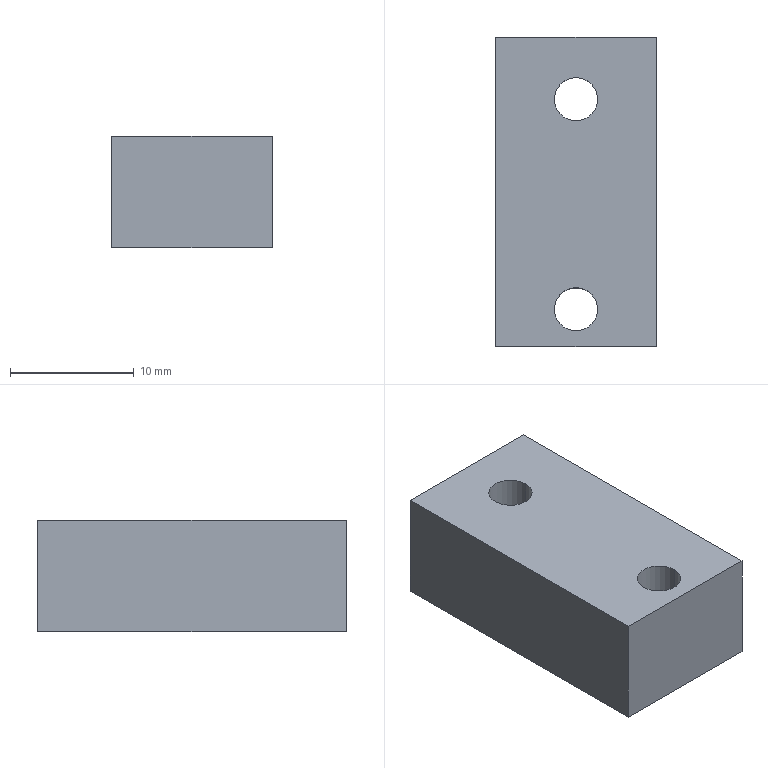Part | SolidWorks | features BaseBody 1 | 1 solid | 10 faces | box 13 x 25 x 9 mm | volume 2752 mm3 | plane 6 | cylinder 4 | commonest cylinder face diameters 3.5 x4
STEP:
#1=CARTESIAN_POINT('',(-21.75,14.,0.));
#2=VERTEX_POINT('',#1);
#3=CARTESIAN_POINT('',(-18.25,14.,0.));
#4=VERTEX_POINT('',#3);
#5=CARTESIAN_POINT('',(-20.,14.,0.));
#6=DIRECTION('',(0.,0.,1.));
#7=DIRECTION('',(1.,0.,0.));
#8=AXIS2_PLACEMENT_3D('',#5,#6,#7);
#9=CIRCLE('',#8,1.75);
#10=EDGE_CURVE('',#2,#4,#9,.T.);
#11=ORIENTED_EDGE('',*,*,#10,.F.);
#12=CARTESIAN_POINT('',(-21.75,14.,9.));
#13=VERTEX_POINT('',#12);
#14=CARTESIAN_POINT('',(-21.75,14.,-20.58));
#15=DIRECTION('',(0.,0.,1.));
#16=VECTOR('',#15,1000.);
#17=LINE('',#14,#16);
#18=EDGE_CURVE('',#2,#13,#17,.T.);
#19=ORIENTED_EDGE('',*,*,#18,.T.);
#20=CARTESIAN_POINT('',(-18.25,14.,9.));
#21=VERTEX_POINT('',#20);
#22=CARTESIAN_POINT('',(-20.,14.,9.));
#23=DIRECTION('',(0.,0.,-1.));
#24=DIRECTION('',(1.,0.,0.));
#25=AXIS2_PLACEMENT_3D('',#22,#23,#24);
#26=CIRCLE('',#25,1.75);
#27=EDGE_CURVE('',#21,#13,#26,.T.);
#28=ORIENTED_EDGE('',*,*,#27,.F.);
#29=CARTESIAN_POINT('',(-18.25,14.,-20.58));
#30=DIRECTION('',(0.,0.,1.));
#31=VECTOR('',#30,1000.);
#32=LINE('',#29,#31);
#33=EDGE_CURVE('',#4,#21,#32,.T.);
#34=ORIENTED_EDGE('',*,*,#33,.F.);
#35=EDGE_LOOP('',(#11,#19,#28,#34));
#36=FACE_OUTER_BOUND('',#35,.T.);
#37=CARTESIAN_POINT('',(-20.,14.,-20.58));
#38=DIRECTION('',(0.,0.,1.));
#39=DIRECTION('',(1.,0.,0.));
#40=AXIS2_PLACEMENT_3D('',#37,#38,#39);
#41=CYLINDRICAL_SURFACE('',#40,1.75);
#42=ADVANCED_FACE('',(#36),#41,.F.);
#43=CARTESIAN_POINT('',(-21.75,-3.,0.));
#44=VERTEX_POINT('',#43);
#45=CARTESIAN_POINT('',(-18.25,-3.,0.));
#46=VERTEX_POINT('',#45);
#47=CARTESIAN_POINT('',(-20.,-3.,0.));
#48=DIRECTION('',(0.,0.,1.));
#49=DIRECTION('',(1.,0.,0.));
#50=AXIS2_PLACEMENT_3D('',#47,#48,#49);
#51=CIRCLE('',#50,1.75);
#52=EDGE_CURVE('',#44,#46,#51,.T.);
#53=ORIENTED_EDGE('',*,*,#52,.F.);
#54=CARTESIAN_POINT('',(-21.75,-3.,9.));
#55=VERTEX_POINT('',#54);
#56=CARTESIAN_POINT('',(-21.75,-3.,-20.58));
#57=DIRECTION('',(0.,0.,1.));
#58=VECTOR('',#57,1000.);
#59=LINE('',#56,#58);
#60=EDGE_CURVE('',#44,#55,#59,.T.);
#61=ORIENTED_EDGE('',*,*,#60,.T.);
#62=CARTESIAN_POINT('',(-18.25,-3.,9.));
#63=VERTEX_POINT('',#62);
#64=CARTESIAN_POINT('',(-20.,-3.,9.));
#65=DIRECTION('',(0.,0.,-1.));
#66=DIRECTION('',(1.,0.,0.));
#67=AXIS2_PLACEMENT_3D('',#64,#65,#66);
#68=CIRCLE('',#67,1.75);
#69=EDGE_CURVE('',#63,#55,#68,.T.);
#70=ORIENTED_EDGE('',*,*,#69,.F.);
#71=CARTESIAN_POINT('',(-18.25,-3.,-20.58));
#72=DIRECTION('',(0.,0.,1.));
#73=VECTOR('',#72,1000.);
#74=LINE('',#71,#73);
#75=EDGE_CURVE('',#46,#63,#74,.T.);
#76=ORIENTED_EDGE('',*,*,#75,.F.);
#77=EDGE_LOOP('',(#53,#61,#70,#76));
#78=FACE_OUTER_BOUND('',#77,.T.);
#79=CARTESIAN_POINT('',(-20.,-3.,-20.58));
#80=DIRECTION('',(0.,0.,1.));
#81=DIRECTION('',(1.,0.,0.));
#82=AXIS2_PLACEMENT_3D('',#79,#80,#81);
#83=CYLINDRICAL_SURFACE('',#82,1.75);
#84=ADVANCED_FACE('',(#78),#83,.F.);
#85=ORIENTED_EDGE('',*,*,#27,.T.);
#86=CARTESIAN_POINT('',(-20.,14.,9.));
#87=DIRECTION('',(0.,0.,-1.));
#88=DIRECTION('',(1.,0.,0.));
#89=AXIS2_PLACEMENT_3D('',#86,#87,#88);
#90=CIRCLE('',#89,1.75);
#91=EDGE_CURVE('',#13,#21,#90,.T.);
#92=ORIENTED_EDGE('',*,*,#91,.T.);
#93=EDGE_LOOP('',(#85,#92));
#94=FACE_BOUND('',#93,.T.);
#95=ORIENTED_EDGE('',*,*,#69,.T.);
#96=CARTESIAN_POINT('',(-20.,-3.,9.));
#97=DIRECTION('',(0.,0.,-1.));
#98=DIRECTION('',(1.,0.,0.));
#99=AXIS2_PLACEMENT_3D('',#96,#97,#98);
#100=CIRCLE('',#99,1.75);
#101=EDGE_CURVE('',#55,#63,#100,.T.);
#102=ORIENTED_EDGE('',*,*,#101,.T.);
#103=EDGE_LOOP('',(#95,#102));
#104=FACE_BOUND('',#103,.T.);
#105=CARTESIAN_POINT('',(-13.5,-6.,9.));
#106=VERTEX_POINT('',#105);
#107=CARTESIAN_POINT('',(-13.5,19.,9.));
#108=VERTEX_POINT('',#107);
#109=CARTESIAN_POINT('',(-13.5,6.5,9.));
#110=DIRECTION('',(0.,1.,0.));
#111=VECTOR('',#110,1000.);
#112=LINE('',#109,#111);
#113=EDGE_CURVE('',#106,#108,#112,.T.);
#114=ORIENTED_EDGE('',*,*,#113,.T.);
#115=CARTESIAN_POINT('',(-26.5,19.,9.));
#116=VERTEX_POINT('',#115);
#117=CARTESIAN_POINT('',(-20.,19.,9.));
#118=DIRECTION('',(-1.,0.,0.));
#119=VECTOR('',#118,1000.);
#120=LINE('',#117,#119);
#121=EDGE_CURVE('',#108,#116,#120,.T.);
#122=ORIENTED_EDGE('',*,*,#121,.T.);
#123=CARTESIAN_POINT('',(-26.5,-6.,9.));
#124=VERTEX_POINT('',#123);
#125=CARTESIAN_POINT('',(-26.5,6.5,9.));
#126=DIRECTION('',(0.,-1.,0.));
#127=VECTOR('',#126,1000.);
#128=LINE('',#125,#127);
#129=EDGE_CURVE('',#116,#124,#128,.T.);
#130=ORIENTED_EDGE('',*,*,#129,.T.);
#131=CARTESIAN_POINT('',(-20.,-6.,9.));
#132=DIRECTION('',(1.,0.,0.));
#133=VECTOR('',#132,1000.);
#134=LINE('',#131,#133);
#135=EDGE_CURVE('',#124,#106,#134,.T.);
#136=ORIENTED_EDGE('',*,*,#135,.T.);
#137=EDGE_LOOP('',(#114,#122,#130,#136));
#138=FACE_OUTER_BOUND('',#137,.T.);
#139=CARTESIAN_POINT('',(-20.,6.5,9.));
#140=DIRECTION('',(0.,0.,1.));
#141=DIRECTION('',(1.,0.,0.));
#142=AXIS2_PLACEMENT_3D('',#139,#140,#141);
#143=PLANE('',#142);
#144=ADVANCED_FACE('',(#94,#104,#138),#143,.T.);
#145=ORIENTED_EDGE('',*,*,#18,.F.);
#146=CARTESIAN_POINT('',(-20.,14.,0.));
#147=DIRECTION('',(0.,0.,1.));
#148=DIRECTION('',(1.,0.,0.));
#149=AXIS2_PLACEMENT_3D('',#146,#147,#148);
#150=CIRCLE('',#149,1.75);
#151=EDGE_CURVE('',#4,#2,#150,.T.);
#152=ORIENTED_EDGE('',*,*,#151,.F.);
#153=ORIENTED_EDGE('',*,*,#33,.T.);
#154=ORIENTED_EDGE('',*,*,#91,.F.);
#155=EDGE_LOOP('',(#145,#152,#153,#154));
#156=FACE_OUTER_BOUND('',#155,.T.);
#157=CARTESIAN_POINT('',(-20.,14.,-20.58));
#158=DIRECTION('',(0.,0.,1.));
#159=DIRECTION('',(1.,0.,0.));
#160=AXIS2_PLACEMENT_3D('',#157,#158,#159);
#161=CYLINDRICAL_SURFACE('',#160,1.75);
#162=ADVANCED_FACE('',(#156),#161,.F.);
#163=ORIENTED_EDGE('',*,*,#60,.F.);
#164=CARTESIAN_POINT('',(-20.,-3.,0.));
#165=DIRECTION('',(0.,0.,1.));
#166=DIRECTION('',(1.,0.,0.));
#167=AXIS2_PLACEMENT_3D('',#164,#165,#166);
#168=CIRCLE('',#167,1.75);
#169=EDGE_CURVE('',#46,#44,#168,.T.);
#170=ORIENTED_EDGE('',*,*,#169,.F.);
#171=ORIENTED_EDGE('',*,*,#75,.T.);
#172=ORIENTED_EDGE('',*,*,#101,.F.);
#173=EDGE_LOOP('',(#163,#170,#171,#172));
#174=FACE_OUTER_BOUND('',#173,.T.);
#175=CARTESIAN_POINT('',(-20.,-3.,-20.58));
#176=DIRECTION('',(0.,0.,1.));
#177=DIRECTION('',(1.,0.,0.));
#178=AXIS2_PLACEMENT_3D('',#175,#176,#177);
#179=CYLINDRICAL_SURFACE('',#178,1.75);
#180=ADVANCED_FACE('',(#174),#179,.F.);
#181=CARTESIAN_POINT('',(-13.5,19.,0.));
#182=VERTEX_POINT('',#181);
#183=CARTESIAN_POINT('',(-26.5,19.,0.));
#184=VERTEX_POINT('',#183);
#185=CARTESIAN_POINT('',(-26.5,19.,0.));
#186=DIRECTION('',(-1.,0.,0.));
#187=VECTOR('',#186,1000.);
#188=LINE('',#185,#187);
#189=EDGE_CURVE('',#182,#184,#188,.T.);
#190=ORIENTED_EDGE('',*,*,#189,.T.);
#191=CARTESIAN_POINT('',(-26.5,19.,0.));
#192=DIRECTION('',(0.,0.,1.));
#193=VECTOR('',#192,1000.);
#194=LINE('',#191,#193);
#195=EDGE_CURVE('',#184,#116,#194,.T.);
#196=ORIENTED_EDGE('',*,*,#195,.T.);
#197=ORIENTED_EDGE('',*,*,#121,.F.);
#198=CARTESIAN_POINT('',(-13.5,19.,0.));
#199=DIRECTION('',(0.,0.,-1.));
#200=VECTOR('',#199,1000.);
#201=LINE('',#198,#200);
#202=EDGE_CURVE('',#108,#182,#201,.T.);
#203=ORIENTED_EDGE('',*,*,#202,.T.);
#204=EDGE_LOOP('',(#190,#196,#197,#203));
#205=FACE_OUTER_BOUND('',#204,.T.);
#206=CARTESIAN_POINT('',(-26.5,19.,0.));
#207=DIRECTION('',(0.,1.,0.));
#208=DIRECTION('',(0.,0.,1.));
#209=AXIS2_PLACEMENT_3D('',#206,#207,#208);
#210=PLANE('',#209);
#211=ADVANCED_FACE('',(#205),#210,.T.);
#212=CARTESIAN_POINT('',(-13.5,-6.,0.));
#213=VERTEX_POINT('',#212);
#214=CARTESIAN_POINT('',(-13.5,19.,0.));
#215=DIRECTION('',(0.,1.,0.));
#216=VECTOR('',#215,1000.);
#217=LINE('',#214,#216);
#218=EDGE_CURVE('',#213,#182,#217,.T.);
#219=ORIENTED_EDGE('',*,*,#218,.T.);
#220=ORIENTED_EDGE('',*,*,#202,.F.);
#221=ORIENTED_EDGE('',*,*,#113,.F.);
#222=CARTESIAN_POINT('',(-13.5,-6.,0.));
#223=DIRECTION('',(0.,0.,-1.));
#224=VECTOR('',#223,1000.);
#225=LINE('',#222,#224);
#226=EDGE_CURVE('',#106,#213,#225,.T.);
#227=ORIENTED_EDGE('',*,*,#226,.T.);
#228=EDGE_LOOP('',(#219,#220,#221,#227));
#229=FACE_OUTER_BOUND('',#228,.T.);
#230=CARTESIAN_POINT('',(-13.5,19.,0.));
#231=DIRECTION('',(1.,0.,0.));
#232=DIRECTION('',(0.,0.,-1.));
#233=AXIS2_PLACEMENT_3D('',#230,#231,#232);
#234=PLANE('',#233);
#235=ADVANCED_FACE('',(#229),#234,.T.);
#236=CARTESIAN_POINT('',(-26.5,-6.,0.));
#237=VERTEX_POINT('',#236);
#238=CARTESIAN_POINT('',(-13.5,-6.,0.));
#239=DIRECTION('',(1.,0.,0.));
#240=VECTOR('',#239,1000.);
#241=LINE('',#238,#240);
#242=EDGE_CURVE('',#237,#213,#241,.T.);
#243=ORIENTED_EDGE('',*,*,#242,.T.);
#244=ORIENTED_EDGE('',*,*,#226,.F.);
#245=ORIENTED_EDGE('',*,*,#135,.F.);
#246=CARTESIAN_POINT('',(-26.5,-6.,0.));
#247=DIRECTION('',(0.,0.,-1.));
#248=VECTOR('',#247,1000.);
#249=LINE('',#246,#248);
#250=EDGE_CURVE('',#124,#237,#249,.T.);
#251=ORIENTED_EDGE('',*,*,#250,.T.);
#252=EDGE_LOOP('',(#243,#244,#245,#251));
#253=FACE_OUTER_BOUND('',#252,.T.);
#254=CARTESIAN_POINT('',(-13.5,-6.,0.));
#255=DIRECTION('',(0.,-1.,0.));
#256=DIRECTION('',(0.,0.,-1.));
#257=AXIS2_PLACEMENT_3D('',#254,#255,#256);
#258=PLANE('',#257);
#259=ADVANCED_FACE('',(#253),#258,.T.);
#260=CARTESIAN_POINT('',(-26.5,-6.,0.));
#261=DIRECTION('',(0.,-1.,0.));
#262=VECTOR('',#261,1000.);
#263=LINE('',#260,#262);
#264=EDGE_CURVE('',#184,#237,#263,.T.);
#265=ORIENTED_EDGE('',*,*,#264,.T.);
#266=ORIENTED_EDGE('',*,*,#250,.F.);
#267=ORIENTED_EDGE('',*,*,#129,.F.);
#268=ORIENTED_EDGE('',*,*,#195,.F.);
#269=EDGE_LOOP('',(#265,#266,#267,#268));
#270=FACE_OUTER_BOUND('',#269,.T.);
#271=CARTESIAN_POINT('',(-26.5,-6.,0.));
#272=DIRECTION('',(-1.,0.,0.));
#273=DIRECTION('',(0.,0.,1.));
#274=AXIS2_PLACEMENT_3D('',#271,#272,#273);
#275=PLANE('',#274);
#276=ADVANCED_FACE('',(#270),#275,.T.);
#277=ORIENTED_EDGE('',*,*,#151,.T.);
#278=ORIENTED_EDGE('',*,*,#10,.T.);
#279=EDGE_LOOP('',(#277,#278));
#280=FACE_BOUND('',#279,.T.);
#281=ORIENTED_EDGE('',*,*,#169,.T.);
#282=ORIENTED_EDGE('',*,*,#52,.T.);
#283=EDGE_LOOP('',(#281,#282));
#284=FACE_BOUND('',#283,.T.);
#285=ORIENTED_EDGE('',*,*,#264,.F.);
#286=ORIENTED_EDGE('',*,*,#189,.F.);
#287=ORIENTED_EDGE('',*,*,#218,.F.);
#288=ORIENTED_EDGE('',*,*,#242,.F.);
#289=EDGE_LOOP('',(#285,#286,#287,#288));
#290=FACE_OUTER_BOUND('',#289,.T.);
#291=CARTESIAN_POINT('',(-20.,6.5,0.));
#292=DIRECTION('',(0.,0.,1.));
#293=DIRECTION('',(1.,0.,0.));
#294=AXIS2_PLACEMENT_3D('',#291,#292,#293);
#295=PLANE('',#294);
#296=ADVANCED_FACE('',(#280,#284,#290),#295,.F.);
#297=CLOSED_SHELL('',(#42,#84,#144,#162,#180,#211,#235,#259,#276,#296));
#298=MANIFOLD_SOLID_BREP('',#297);
#299=CARTESIAN_POINT('',(0.,0.,0.));
#300=DIRECTION('',(0.,0.,1.));
#301=DIRECTION('',(1.,0.,0.));
#302=AXIS2_PLACEMENT_3D('',#299,#300,#301);
#303=(LENGTH_UNIT()NAMED_UNIT(*)SI_UNIT(.MILLI.,.METRE.));
#304=UNCERTAINTY_MEASURE_WITH_UNIT(LENGTH_MEASURE(0.00001),#303,'','');
#305=(NAMED_UNIT(*)PLANE_ANGLE_UNIT()SI_UNIT($,.RADIAN.));
#306=(NAMED_UNIT(*)SI_UNIT($,.STERADIAN.)SOLID_ANGLE_UNIT());
#307=(GEOMETRIC_REPRESENTATION_CONTEXT(3)GLOBAL_UNCERTAINTY_ASSIGNED_CONTEXT((#304))GLOBAL_UNIT_ASSIGNED_CONTEXT((#303,#305,#306))REPRESENTATION_CONTEXT('',''));
#308=ADVANCED_BREP_SHAPE_REPRESENTATION('',(#298,#302),#307);